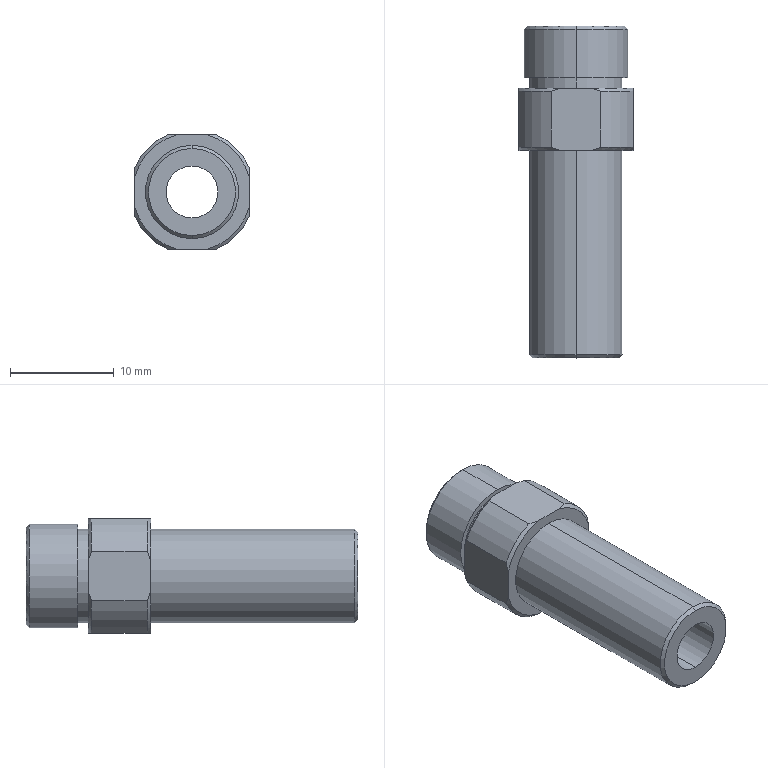Part | SolidWorks | features Chamfer 5, ICE 4, HoleWzd 3, RevCut 2, Extrusion 1 | 1 solid | 33 faces | box 11 x 32 x 11 mm | volume 1736 mm3 | cone 12 | cylinder 12 | plane 9 | commonest cylinder face diameters 9 x4 12 x4 5 x2 10 x2
STEP:
#1=CARTESIAN_POINT('',(0.,-32.,-4.2));
#2=VERTEX_POINT('',#1);
#3=CARTESIAN_POINT('',(0.,-32.,4.2));
#4=VERTEX_POINT('',#3);
#5=CARTESIAN_POINT('',(0.,-32.,0.));
#6=DIRECTION('',(0.,-1.,0.));
#7=DIRECTION('',(0.,0.,-1.));
#8=AXIS2_PLACEMENT_3D('',#5,#6,#7);
#9=CIRCLE('',#8,4.2);
#10=EDGE_CURVE('',#2,#4,#9,.T.);
#11=ORIENTED_EDGE('',*,*,#10,.F.);
#12=CARTESIAN_POINT('',(0.,-31.7,-4.5));
#13=VERTEX_POINT('',#12);
#14=CARTESIAN_POINT('',(0.,-32.,-4.2));
#15=DIRECTION('',(0.,0.7071,-0.7071));
#16=VECTOR('',#15,1000.);
#17=LINE('',#14,#16);
#18=EDGE_CURVE('',#2,#13,#17,.T.);
#19=ORIENTED_EDGE('',*,*,#18,.T.);
#20=CARTESIAN_POINT('',(0.,-31.7,4.5));
#21=VERTEX_POINT('',#20);
#22=CARTESIAN_POINT('',(0.,-31.7,0.));
#23=DIRECTION('',(0.,1.,0.));
#24=DIRECTION('',(0.,0.,-1.));
#25=AXIS2_PLACEMENT_3D('',#22,#23,#24);
#26=CIRCLE('',#25,4.5);
#27=EDGE_CURVE('',#21,#13,#26,.T.);
#28=ORIENTED_EDGE('',*,*,#27,.F.);
#29=CARTESIAN_POINT('',(0.,-32.,4.2));
#30=DIRECTION('',(0.,0.7071,0.7071));
#31=VECTOR('',#30,1000.);
#32=LINE('',#29,#31);
#33=EDGE_CURVE('',#4,#21,#32,.T.);
#34=ORIENTED_EDGE('',*,*,#33,.F.);
#35=EDGE_LOOP('',(#11,#19,#28,#34));
#36=FACE_OUTER_BOUND('',#35,.T.);
#37=CARTESIAN_POINT('',(0.,-32.,0.));
#38=DIRECTION('',(0.,1.,0.));
#39=DIRECTION('',(0.,0.,1.));
#40=AXIS2_PLACEMENT_3D('',#37,#38,#39);
#41=CONICAL_SURFACE('',#40,4.2,0.7854);
#42=ADVANCED_FACE('',(#36),#41,.T.);
#43=CARTESIAN_POINT('',(0.,-5.,-4.5));
#44=VERTEX_POINT('',#43);
#45=CARTESIAN_POINT('',(0.,-5.,4.5));
#46=VERTEX_POINT('',#45);
#47=CARTESIAN_POINT('',(0.,-5.,0.));
#48=DIRECTION('',(0.,-1.,0.));
#49=DIRECTION('',(0.,0.,-1.));
#50=AXIS2_PLACEMENT_3D('',#47,#48,#49);
#51=CIRCLE('',#50,4.5);
#52=EDGE_CURVE('',#44,#46,#51,.T.);
#53=ORIENTED_EDGE('',*,*,#52,.T.);
#54=CARTESIAN_POINT('',(0.,-6.,4.5));
#55=VERTEX_POINT('',#54);
#56=CARTESIAN_POINT('',(0.,-6.,4.5));
#57=DIRECTION('',(0.,-1.,0.));
#58=VECTOR('',#57,1000.);
#59=LINE('',#56,#58);
#60=EDGE_CURVE('',#46,#55,#59,.T.);
#61=ORIENTED_EDGE('',*,*,#60,.T.);
#62=CARTESIAN_POINT('',(0.,-6.,-4.5));
#63=VERTEX_POINT('',#62);
#64=CARTESIAN_POINT('',(0.,-6.,0.));
#65=DIRECTION('',(0.,-1.,0.));
#66=DIRECTION('',(0.,0.,-1.));
#67=AXIS2_PLACEMENT_3D('',#64,#65,#66);
#68=CIRCLE('',#67,4.5);
#69=EDGE_CURVE('',#63,#55,#68,.T.);
#70=ORIENTED_EDGE('',*,*,#69,.F.);
#71=CARTESIAN_POINT('',(0.,-6.,-4.5));
#72=DIRECTION('',(0.,-1.,0.));
#73=VECTOR('',#72,1000.);
#74=LINE('',#71,#73);
#75=EDGE_CURVE('',#44,#63,#74,.T.);
#76=ORIENTED_EDGE('',*,*,#75,.F.);
#77=EDGE_LOOP('',(#53,#61,#70,#76));
#78=FACE_OUTER_BOUND('',#77,.T.);
#79=CARTESIAN_POINT('',(0.,-6.,0.));
#80=DIRECTION('',(0.,-1.,0.));
#81=DIRECTION('',(0.,0.,-1.));
#82=AXIS2_PLACEMENT_3D('',#79,#80,#81);
#83=CYLINDRICAL_SURFACE('',#82,4.5);
#84=ADVANCED_FACE('',(#78),#83,.T.);
#85=CARTESIAN_POINT('',(0.,-32.,2.5));
#86=VERTEX_POINT('',#85);
#87=CARTESIAN_POINT('',(0.,-32.,-2.5));
#88=VERTEX_POINT('',#87);
#89=CARTESIAN_POINT('',(0.,-32.,0.));
#90=DIRECTION('',(0.,-1.,0.));
#91=DIRECTION('',(0.,0.,-1.));
#92=AXIS2_PLACEMENT_3D('',#89,#90,#91);
#93=CIRCLE('',#92,2.5);
#94=EDGE_CURVE('',#86,#88,#93,.T.);
#95=ORIENTED_EDGE('',*,*,#94,.T.);
#96=CARTESIAN_POINT('',(0.,0.,-2.5));
#97=VERTEX_POINT('',#96);
#98=CARTESIAN_POINT('',(0.,0.,-2.5));
#99=DIRECTION('',(0.,1.,0.));
#100=VECTOR('',#99,1000.);
#101=LINE('',#98,#100);
#102=EDGE_CURVE('',#88,#97,#101,.T.);
#103=ORIENTED_EDGE('',*,*,#102,.T.);
#104=CARTESIAN_POINT('',(0.,0.,2.5));
#105=VERTEX_POINT('',#104);
#106=CARTESIAN_POINT('',(0.,0.,0.));
#107=DIRECTION('',(0.,1.,0.));
#108=DIRECTION('',(0.,0.,1.));
#109=AXIS2_PLACEMENT_3D('',#106,#107,#108);
#110=CIRCLE('',#109,2.5);
#111=EDGE_CURVE('',#97,#105,#110,.T.);
#112=ORIENTED_EDGE('',*,*,#111,.T.);
#113=CARTESIAN_POINT('',(0.,0.,2.5));
#114=DIRECTION('',(0.,1.,0.));
#115=VECTOR('',#114,1000.);
#116=LINE('',#113,#115);
#117=EDGE_CURVE('',#86,#105,#116,.T.);
#118=ORIENTED_EDGE('',*,*,#117,.F.);
#119=EDGE_LOOP('',(#95,#103,#112,#118));
#120=FACE_OUTER_BOUND('',#119,.T.);
#121=CARTESIAN_POINT('',(0.,0.,0.));
#122=DIRECTION('',(0.,1.,0.));
#123=DIRECTION('',(0.,0.,1.));
#124=AXIS2_PLACEMENT_3D('',#121,#122,#123);
#125=CYLINDRICAL_SURFACE('',#124,2.5);
#126=ADVANCED_FACE('',(#120),#125,.F.);
#127=CARTESIAN_POINT('',(0.,0.,4.7));
#128=VERTEX_POINT('',#127);
#129=CARTESIAN_POINT('',(0.,0.,-4.7));
#130=VERTEX_POINT('',#129);
#131=CARTESIAN_POINT('',(0.,0.,0.));
#132=DIRECTION('',(0.,1.,0.));
#133=DIRECTION('',(0.,0.,1.));
#134=AXIS2_PLACEMENT_3D('',#131,#132,#133);
#135=CIRCLE('',#134,4.7);
#136=EDGE_CURVE('',#128,#130,#135,.T.);
#137=ORIENTED_EDGE('',*,*,#136,.F.);
#138=CARTESIAN_POINT('',(0.,-0.3,5.));
#139=VERTEX_POINT('',#138);
#140=CARTESIAN_POINT('',(0.,0.,4.7));
#141=DIRECTION('',(0.,-0.7071,0.7071));
#142=VECTOR('',#141,1000.);
#143=LINE('',#140,#142);
#144=EDGE_CURVE('',#128,#139,#143,.T.);
#145=ORIENTED_EDGE('',*,*,#144,.T.);
#146=CARTESIAN_POINT('',(0.,-0.3,-5.));
#147=VERTEX_POINT('',#146);
#148=CARTESIAN_POINT('',(0.,-0.3,0.));
#149=DIRECTION('',(0.,-1.,0.));
#150=DIRECTION('',(0.,0.,1.));
#151=AXIS2_PLACEMENT_3D('',#148,#149,#150);
#152=CIRCLE('',#151,5.);
#153=EDGE_CURVE('',#147,#139,#152,.T.);
#154=ORIENTED_EDGE('',*,*,#153,.F.);
#155=CARTESIAN_POINT('',(0.,0.,-4.7));
#156=DIRECTION('',(0.,-0.7071,-0.7071));
#157=VECTOR('',#156,1000.);
#158=LINE('',#155,#157);
#159=EDGE_CURVE('',#130,#147,#158,.T.);
#160=ORIENTED_EDGE('',*,*,#159,.F.);
#161=EDGE_LOOP('',(#137,#145,#154,#160));
#162=FACE_OUTER_BOUND('',#161,.T.);
#163=CARTESIAN_POINT('',(0.,0.,0.));
#164=DIRECTION('',(0.,-1.,0.));
#165=DIRECTION('',(0.,0.,-1.));
#166=AXIS2_PLACEMENT_3D('',#163,#164,#165);
#167=CONICAL_SURFACE('',#166,4.7,0.7854);
#168=ADVANCED_FACE('',(#162),#167,.T.);
#169=ORIENTED_EDGE('',*,*,#27,.T.);
#170=CARTESIAN_POINT('',(0.,-12.,-4.5));
#171=VERTEX_POINT('',#170);
#172=CARTESIAN_POINT('',(0.,-32.,-4.5));
#173=DIRECTION('',(0.,1.,0.));
#174=VECTOR('',#173,1000.);
#175=LINE('',#172,#174);
#176=EDGE_CURVE('',#13,#171,#175,.T.);
#177=ORIENTED_EDGE('',*,*,#176,.T.);
#178=CARTESIAN_POINT('',(0.,-12.,4.5));
#179=VERTEX_POINT('',#178);
#180=CARTESIAN_POINT('',(0.,-12.,0.));
#181=DIRECTION('',(0.,-1.,0.));
#182=DIRECTION('',(0.,0.,-1.));
#183=AXIS2_PLACEMENT_3D('',#180,#181,#182);
#184=CIRCLE('',#183,4.5);
#185=EDGE_CURVE('',#171,#179,#184,.T.);
#186=ORIENTED_EDGE('',*,*,#185,.T.);
#187=CARTESIAN_POINT('',(0.,-32.,4.5));
#188=DIRECTION('',(0.,1.,0.));
#189=VECTOR('',#188,1000.);
#190=LINE('',#187,#189);
#191=EDGE_CURVE('',#21,#179,#190,.T.);
#192=ORIENTED_EDGE('',*,*,#191,.F.);
#193=EDGE_LOOP('',(#169,#177,#186,#192));
#194=FACE_OUTER_BOUND('',#193,.T.);
#195=CARTESIAN_POINT('',(0.,-32.,0.));
#196=DIRECTION('',(0.,1.,0.));
#197=DIRECTION('',(0.,0.,1.));
#198=AXIS2_PLACEMENT_3D('',#195,#196,#197);
#199=CYLINDRICAL_SURFACE('',#198,4.5);
#200=ADVANCED_FACE('',(#194),#199,.T.);
#201=CARTESIAN_POINT('',(0.,-5.,5.));
#202=VERTEX_POINT('',#201);
#203=CARTESIAN_POINT('',(0.,-5.,-5.));
#204=VERTEX_POINT('',#203);
#205=CARTESIAN_POINT('',(0.,-5.,0.));
#206=DIRECTION('',(0.,1.,0.));
#207=DIRECTION('',(0.,0.,-1.));
#208=AXIS2_PLACEMENT_3D('',#205,#206,#207);
#209=CIRCLE('',#208,5.);
#210=EDGE_CURVE('',#202,#204,#209,.T.);
#211=ORIENTED_EDGE('',*,*,#210,.T.);
#212=CARTESIAN_POINT('',(0.,-6.,-5.));
#213=DIRECTION('',(0.,1.,0.));
#214=VECTOR('',#213,1000.);
#215=LINE('',#212,#214);
#216=EDGE_CURVE('',#204,#147,#215,.T.);
#217=ORIENTED_EDGE('',*,*,#216,.T.);
#218=ORIENTED_EDGE('',*,*,#153,.T.);
#219=CARTESIAN_POINT('',(0.,-6.,5.));
#220=DIRECTION('',(0.,1.,0.));
#221=VECTOR('',#220,1000.);
#222=LINE('',#219,#221);
#223=EDGE_CURVE('',#202,#139,#222,.T.);
#224=ORIENTED_EDGE('',*,*,#223,.F.);
#225=EDGE_LOOP('',(#211,#217,#218,#224));
#226=FACE_OUTER_BOUND('',#225,.T.);
#227=CARTESIAN_POINT('',(0.,-6.,0.));
#228=DIRECTION('',(0.,1.,0.));
#229=DIRECTION('',(0.,0.,1.));
#230=AXIS2_PLACEMENT_3D('',#227,#228,#229);
#231=CYLINDRICAL_SURFACE('',#230,5.);
#232=ADVANCED_FACE('',(#226),#231,.T.);
#233=CARTESIAN_POINT('',(-2.398,-6.3,-5.5));
#234=VERTEX_POINT('',#233);
#235=CARTESIAN_POINT('',(-1.497,-6.,-5.5));
#236=VERTEX_POINT('',#235);
#237=CARTESIAN_POINT('',(-2.398,-6.3,-5.5));
#238=CARTESIAN_POINT('',(-2.104,-6.182,-5.5));
#239=CARTESIAN_POINT('',(-1.804,-6.081,-5.5));
#240=CARTESIAN_POINT('',(-1.497,-6.,-5.5));
#241=B_SPLINE_CURVE_WITH_KNOTS('',3,(#237,#238,#239,#240),.UNSPECIFIED.,.F.,.F.,(4,4),(0.01116,0.01211),.UNSPECIFIED.);
#242=EDGE_CURVE('',#234,#236,#241,.T.);
#243=ORIENTED_EDGE('',*,*,#242,.F.);
#244=CARTESIAN_POINT('',(-5.5,-6.3,-2.398));
#245=VERTEX_POINT('',#244);
#246=CARTESIAN_POINT('',(0.,-6.3,0.));
#247=DIRECTION('',(0.,-1.,0.));
#248=DIRECTION('',(0.,0.,-1.));
#249=AXIS2_PLACEMENT_3D('',#246,#247,#248);
#250=CIRCLE('',#249,6.);
#251=EDGE_CURVE('',#245,#234,#250,.T.);
#252=ORIENTED_EDGE('',*,*,#251,.F.);
#253=CARTESIAN_POINT('',(-5.5,-6.,-1.497));
#254=VERTEX_POINT('',#253);
#255=CARTESIAN_POINT('',(-5.5,-6.,-1.497));
#256=CARTESIAN_POINT('',(-5.5,-6.08,-1.802));
#257=CARTESIAN_POINT('',(-5.5,-6.182,-2.102));
#258=CARTESIAN_POINT('',(-5.5,-6.3,-2.398));
#259=B_SPLINE_CURVE_WITH_KNOTS('',3,(#255,#256,#257,#258),.UNSPECIFIED.,.F.,.F.,(4,4),(0.01603,0.01698),.UNSPECIFIED.);
#260=EDGE_CURVE('',#254,#245,#259,.T.);
#261=ORIENTED_EDGE('',*,*,#260,.F.);
#262=CARTESIAN_POINT('',(0.,-6.,0.));
#263=DIRECTION('',(0.,1.,0.));
#264=DIRECTION('',(0.,0.,-1.));
#265=AXIS2_PLACEMENT_3D('',#262,#263,#264);
#266=CIRCLE('',#265,5.7);
#267=EDGE_CURVE('',#236,#254,#266,.T.);
#268=ORIENTED_EDGE('',*,*,#267,.F.);
#269=EDGE_LOOP('',(#243,#252,#261,#268));
#270=FACE_OUTER_BOUND('',#269,.T.);
#271=CARTESIAN_POINT('',(0.,-6.3,0.));
#272=DIRECTION('',(0.,-1.,0.));
#273=DIRECTION('',(0.,0.,-1.));
#274=AXIS2_PLACEMENT_3D('',#271,#272,#273);
#275=CONICAL_SURFACE('',#274,6.,0.7854);
#276=ADVANCED_FACE('',(#270),#275,.T.);
#277=CARTESIAN_POINT('',(5.5,-11.7,-2.398));
#278=VERTEX_POINT('',#277);
#279=CARTESIAN_POINT('',(2.398,-11.7,-5.5));
#280=VERTEX_POINT('',#279);
#281=CARTESIAN_POINT('',(0.,-11.7,0.));
#282=DIRECTION('',(0.,1.,0.));
#283=DIRECTION('',(0.,0.,-1.));
#284=AXIS2_PLACEMENT_3D('',#281,#282,#283);
#285=CIRCLE('',#284,6.);
#286=EDGE_CURVE('',#278,#280,#285,.T.);
#287=ORIENTED_EDGE('',*,*,#286,.T.);
#288=CARTESIAN_POINT('',(2.398,-6.3,-5.5));
#289=VERTEX_POINT('',#288);
#290=CARTESIAN_POINT('',(2.398,-12.,-5.5));
#291=DIRECTION('',(0.,1.,0.));
#292=VECTOR('',#291,1000.);
#293=LINE('',#290,#292);
#294=EDGE_CURVE('',#280,#289,#293,.T.);
#295=ORIENTED_EDGE('',*,*,#294,.T.);
#296=CARTESIAN_POINT('',(5.5,-6.3,-2.398));
#297=VERTEX_POINT('',#296);
#298=CARTESIAN_POINT('',(0.,-6.3,0.));
#299=DIRECTION('',(0.,-1.,0.));
#300=DIRECTION('',(0.,0.,-1.));
#301=AXIS2_PLACEMENT_3D('',#298,#299,#300);
#302=CIRCLE('',#301,6.);
#303=EDGE_CURVE('',#289,#297,#302,.T.);
#304=ORIENTED_EDGE('',*,*,#303,.T.);
#305=CARTESIAN_POINT('',(5.5,-12.,-2.398));
#306=DIRECTION('',(0.,-1.,0.));
#307=VECTOR('',#306,1000.);
#308=LINE('',#305,#307);
#309=EDGE_CURVE('',#297,#278,#308,.T.);
#310=ORIENTED_EDGE('',*,*,#309,.T.);
#311=EDGE_LOOP('',(#287,#295,#304,#310));
#312=FACE_OUTER_BOUND('',#311,.T.);
#313=CARTESIAN_POINT('',(0.,-12.,0.));
#314=DIRECTION('',(0.,1.,0.));
#315=DIRECTION('',(0.,0.,1.));
#316=AXIS2_PLACEMENT_3D('',#313,#314,#315);
#317=CYLINDRICAL_SURFACE('',#316,6.);
#318=ADVANCED_FACE('',(#312),#317,.T.);
#319=CARTESIAN_POINT('',(1.497,-12.,-5.5));
#320=VERTEX_POINT('',#319);
#321=CARTESIAN_POINT('',(2.398,-11.7,-5.5));
#322=CARTESIAN_POINT('',(2.104,-11.818,-5.5));
#323=CARTESIAN_POINT('',(1.804,-11.919,-5.5));
#324=CARTESIAN_POINT('',(1.497,-12.,-5.5));
#325=B_SPLINE_CURVE_WITH_KNOTS('',3,(#321,#322,#323,#324),.UNSPECIFIED.,.F.,.F.,(4,4),(0.01116,0.01211),.UNSPECIFIED.);
#326=EDGE_CURVE('',#280,#320,#325,.T.);
#327=ORIENTED_EDGE('',*,*,#326,.F.);
#328=ORIENTED_EDGE('',*,*,#286,.F.);
#329=CARTESIAN_POINT('',(5.5,-12.,-1.497));
#330=VERTEX_POINT('',#329);
#331=CARTESIAN_POINT('',(5.5,-12.,-1.497));
#332=CARTESIAN_POINT('',(5.5,-11.92,-1.802));
#333=CARTESIAN_POINT('',(5.5,-11.818,-2.102));
#334=CARTESIAN_POINT('',(5.5,-11.7,-2.398));
#335=B_SPLINE_CURVE_WITH_KNOTS('',3,(#331,#332,#333,#334),.UNSPECIFIED.,.F.,.F.,(4,4),(0.01603,0.01698),.UNSPECIFIED.);
#336=EDGE_CURVE('',#330,#278,#335,.T.);
#337=ORIENTED_EDGE('',*,*,#336,.F.);
#338=CARTESIAN_POINT('',(0.,-12.,0.));
#339=DIRECTION('',(0.,-1.,0.));
#340=DIRECTION('',(0.,0.,-1.));
#341=AXIS2_PLACEMENT_3D('',#338,#339,#340);
#342=CIRCLE('',#341,5.7);
#343=EDGE_CURVE('',#320,#330,#342,.T.);
#344=ORIENTED_EDGE('',*,*,#343,.F.);
#345=EDGE_LOOP('',(#327,#328,#337,#344));
#346=FACE_OUTER_BOUND('',#345,.T.);
#347=CARTESIAN_POINT('',(0.,-12.,0.));
#348=DIRECTION('',(0.,1.,0.));
#349=DIRECTION('',(0.,0.,1.));
#350=AXIS2_PLACEMENT_3D('',#347,#348,#349);
#351=CONICAL_SURFACE('',#350,5.7,0.7854);
#352=ADVANCED_FACE('',(#346),#351,.T.);
#353=CARTESIAN_POINT('',(-5.5,-11.7,2.398));
#354=VERTEX_POINT('',#353);
#355=CARTESIAN_POINT('',(-2.398,-11.7,5.5));
#356=VERTEX_POINT('',#355);
#357=CARTESIAN_POINT('',(0.,-11.7,0.));
#358=DIRECTION('',(0.,1.,0.));
#359=DIRECTION('',(0.,0.,-1.));
#360=AXIS2_PLACEMENT_3D('',#357,#358,#359);
#361=CIRCLE('',#360,6.);
#362=EDGE_CURVE('',#354,#356,#361,.T.);
#363=ORIENTED_EDGE('',*,*,#362,.T.);
#364=CARTESIAN_POINT('',(-2.398,-6.3,5.5));
#365=VERTEX_POINT('',#364);
#366=CARTESIAN_POINT('',(-2.398,-12.,5.5));
#367=DIRECTION('',(0.,1.,0.));
#368=VECTOR('',#367,1000.);
#369=LINE('',#366,#368);
#370=EDGE_CURVE('',#356,#365,#369,.T.);
#371=ORIENTED_EDGE('',*,*,#370,.T.);
#372=CARTESIAN_POINT('',(-5.5,-6.3,2.398));
#373=VERTEX_POINT('',#372);
#374=CARTESIAN_POINT('',(0.,-6.3,0.));
#375=DIRECTION('',(0.,-1.,0.));
#376=DIRECTION('',(0.,0.,-1.));
#377=AXIS2_PLACEMENT_3D('',#374,#375,#376);
#378=CIRCLE('',#377,6.);
#379=EDGE_CURVE('',#365,#373,#378,.T.);
#380=ORIENTED_EDGE('',*,*,#379,.T.);
#381=CARTESIAN_POINT('',(-5.5,-12.,2.398));
#382=DIRECTION('',(0.,-1.,0.));
#383=VECTOR('',#382,1000.);
#384=LINE('',#381,#383);
#385=EDGE_CURVE('',#373,#354,#384,.T.);
#386=ORIENTED_EDGE('',*,*,#385,.T.);
#387=EDGE_LOOP('',(#363,#371,#380,#386));
#388=FACE_OUTER_BOUND('',#387,.T.);
#389=CARTESIAN_POINT('',(0.,-12.,0.));
#390=DIRECTION('',(0.,1.,0.));
#391=DIRECTION('',(0.,0.,1.));
#392=AXIS2_PLACEMENT_3D('',#389,#390,#391);
#393=CYLINDRICAL_SURFACE('',#392,6.);
#394=ADVANCED_FACE('',(#388),#393,.T.);
#395=CARTESIAN_POINT('',(-1.497,-12.,5.5));
#396=VERTEX_POINT('',#395);
#397=CARTESIAN_POINT('',(-2.398,-11.7,5.5));
#398=CARTESIAN_POINT('',(-2.104,-11.818,5.5));
#399=CARTESIAN_POINT('',(-1.804,-11.919,5.5));
#400=CARTESIAN_POINT('',(-1.497,-12.,5.5));
#401=B_SPLINE_CURVE_WITH_KNOTS('',3,(#397,#398,#399,#400),.UNSPECIFIED.,.F.,.F.,(4,4),(0.01116,0.01211),.UNSPECIFIED.);
#402=EDGE_CURVE('',#356,#396,#401,.T.);
#403=ORIENTED_EDGE('',*,*,#402,.F.);
#404=ORIENTED_EDGE('',*,*,#362,.F.);
#405=CARTESIAN_POINT('',(-5.5,-12.,1.497));
#406=VERTEX_POINT('',#405);
#407=CARTESIAN_POINT('',(-5.5,-12.,1.497));
#408=CARTESIAN_POINT('',(-5.5,-11.92,1.802));
#409=CARTESIAN_POINT('',(-5.5,-11.818,2.102));
#410=CARTESIAN_POINT('',(-5.5,-11.7,2.398));
#411=B_SPLINE_CURVE_WITH_KNOTS('',3,(#407,#408,#409,#410),.UNSPECIFIED.,.F.,.F.,(4,4),(0.01603,0.01698),.UNSPECIFIED.);
#412=EDGE_CURVE('',#406,#354,#411,.T.);
#413=ORIENTED_EDGE('',*,*,#412,.F.);
#414=CARTESIAN_POINT('',(0.,-12.,0.));
#415=DIRECTION('',(0.,-1.,0.));
#416=DIRECTION('',(0.,0.,-1.));
#417=AXIS2_PLACEMENT_3D('',#414,#415,#416);
#418=CIRCLE('',#417,5.7);
#419=EDGE_CURVE('',#396,#406,#418,.T.);
#420=ORIENTED_EDGE('',*,*,#419,.F.);
#421=EDGE_LOOP('',(#403,#404,#413,#420));
#422=FACE_OUTER_BOUND('',#421,.T.);
#423=CARTESIAN_POINT('',(0.,-12.,0.));
#424=DIRECTION('',(0.,1.,0.));
#425=DIRECTION('',(0.,0.,1.));
#426=AXIS2_PLACEMENT_3D('',#423,#424,#425);
#427=CONICAL_SURFACE('',#426,5.7,0.7854);
#428=ADVANCED_FACE('',(#422),#427,.T.);
#429=CARTESIAN_POINT('',(2.398,-6.3,5.5));
#430=VERTEX_POINT('',#429);
#431=CARTESIAN_POINT('',(1.497,-6.,5.5));
#432=VERTEX_POINT('',#431);
#433=CARTESIAN_POINT('',(2.398,-6.3,5.5));
#434=CARTESIAN_POINT('',(2.104,-6.182,5.5));
#435=CARTESIAN_POINT('',(1.804,-6.081,5.5));
#436=CARTESIAN_POINT('',(1.497,-6.,5.5));
#437=B_SPLINE_CURVE_WITH_KNOTS('',3,(#433,#434,#435,#436),.UNSPECIFIED.,.F.,.F.,(4,4),(0.01116,0.01211),.UNSPECIFIED.);
#438=EDGE_CURVE('',#430,#432,#437,.T.);
#439=ORIENTED_EDGE('',*,*,#438,.F.);
#440=CARTESIAN_POINT('',(5.5,-6.3,2.398));
#441=VERTEX_POINT('',#440);
#442=CARTESIAN_POINT('',(0.,-6.3,0.));
#443=DIRECTION('',(0.,-1.,0.));
#444=DIRECTION('',(0.,0.,-1.));
#445=AXIS2_PLACEMENT_3D('',#442,#443,#444);
#446=CIRCLE('',#445,6.);
#447=EDGE_CURVE('',#441,#430,#446,.T.);
#448=ORIENTED_EDGE('',*,*,#447,.F.);
#449=CARTESIAN_POINT('',(5.5,-6.,1.497));
#450=VERTEX_POINT('',#449);
#451=CARTESIAN_POINT('',(5.5,-6.,1.497));
#452=CARTESIAN_POINT('',(5.5,-6.08,1.802));
#453=CARTESIAN_POINT('',(5.5,-6.182,2.102));
#454=CARTESIAN_POINT('',(5.5,-6.3,2.398));
#455=B_SPLINE_CURVE_WITH_KNOTS('',3,(#451,#452,#453,#454),.UNSPECIFIED.,.F.,.F.,(4,4),(0.01603,0.01698),.UNSPECIFIED.);
#456=EDGE_CURVE('',#450,#441,#455,.T.);
#457=ORIENTED_EDGE('',*,*,#456,.F.);
#458=CARTESIAN_POINT('',(0.,-6.,0.));
#459=DIRECTION('',(0.,1.,0.));
#460=DIRECTION('',(0.,0.,-1.));
#461=AXIS2_PLACEMENT_3D('',#458,#459,#460);
#462=CIRCLE('',#461,5.7);
#463=EDGE_CURVE('',#432,#450,#462,.T.);
#464=ORIENTED_EDGE('',*,*,#463,.F.);
#465=EDGE_LOOP('',(#439,#448,#457,#464));
#466=FACE_OUTER_BOUND('',#465,.T.);
#467=CARTESIAN_POINT('',(0.,-6.3,0.));
#468=DIRECTION('',(0.,-1.,0.));
#469=DIRECTION('',(0.,0.,-1.));
#470=AXIS2_PLACEMENT_3D('',#467,#468,#469);
#471=CONICAL_SURFACE('',#470,6.,0.7854);
#472=ADVANCED_FACE('',(#466),#471,.T.);
#473=ORIENTED_EDGE('',*,*,#216,.F.);
#474=CARTESIAN_POINT('',(0.,-5.,0.));
#475=DIRECTION('',(0.,1.,0.));
#476=DIRECTION('',(0.,0.,-1.));
#477=AXIS2_PLACEMENT_3D('',#474,#475,#476);
#478=CIRCLE('',#477,5.);
#479=EDGE_CURVE('',#204,#202,#478,.T.);
#480=ORIENTED_EDGE('',*,*,#479,.T.);
#481=ORIENTED_EDGE('',*,*,#223,.T.);
#482=CARTESIAN_POINT('',(0.,-0.3,0.));
#483=DIRECTION('',(0.,-1.,0.));
#484=DIRECTION('',(0.,0.,1.));
#485=AXIS2_PLACEMENT_3D('',#482,#483,#484);
#486=CIRCLE('',#485,5.);
#487=EDGE_CURVE('',#139,#147,#486,.T.);
#488=ORIENTED_EDGE('',*,*,#487,.T.);
#489=EDGE_LOOP('',(#473,#480,#481,#488));
#490=FACE_OUTER_BOUND('',#489,.T.);
#491=CARTESIAN_POINT('',(0.,-6.,0.));
#492=DIRECTION('',(0.,1.,0.));
#493=DIRECTION('',(0.,0.,1.));
#494=AXIS2_PLACEMENT_3D('',#491,#492,#493);
#495=CYLINDRICAL_SURFACE('',#494,5.);
#496=ADVANCED_FACE('',(#490),#495,.T.);
#497=ORIENTED_EDGE('',*,*,#447,.T.);
#498=CARTESIAN_POINT('',(2.398,-11.7,5.5));
#499=VERTEX_POINT('',#498);
#500=CARTESIAN_POINT('',(2.398,-12.,5.5));
#501=DIRECTION('',(0.,-1.,0.));
#502=VECTOR('',#501,1000.);
#503=LINE('',#500,#502);
#504=EDGE_CURVE('',#430,#499,#503,.T.);
#505=ORIENTED_EDGE('',*,*,#504,.T.);
#506=CARTESIAN_POINT('',(5.5,-11.7,2.398));
#507=VERTEX_POINT('',#506);
#508=CARTESIAN_POINT('',(0.,-11.7,0.));
#509=DIRECTION('',(0.,1.,0.));
#510=DIRECTION('',(0.,0.,-1.));
#511=AXIS2_PLACEMENT_3D('',#508,#509,#510);
#512=CIRCLE('',#511,6.);
#513=EDGE_CURVE('',#499,#507,#512,.T.);
#514=ORIENTED_EDGE('',*,*,#513,.T.);
#515=CARTESIAN_POINT('',(5.5,-12.,2.398));
#516=DIRECTION('',(0.,1.,0.));
#517=VECTOR('',#516,1000.);
#518=LINE('',#515,#517);
#519=EDGE_CURVE('',#507,#441,#518,.T.);
#520=ORIENTED_EDGE('',*,*,#519,.T.);
#521=EDGE_LOOP('',(#497,#505,#514,#520));
#522=FACE_OUTER_BOUND('',#521,.T.);
#523=CARTESIAN_POINT('',(0.,-12.,0.));
#524=DIRECTION('',(0.,1.,0.));
#525=DIRECTION('',(0.,0.,1.));
#526=AXIS2_PLACEMENT_3D('',#523,#524,#525);
#527=CYLINDRICAL_SURFACE('',#526,6.);
#528=ADVANCED_FACE('',(#522),#527,.T.);
#529=CARTESIAN_POINT('',(1.497,-12.,5.5));
#530=VERTEX_POINT('',#529);
#531=CARTESIAN_POINT('',(1.497,-12.,5.5));
#532=CARTESIAN_POINT('',(1.804,-11.919,5.5));
#533=CARTESIAN_POINT('',(2.104,-11.818,5.5));
#534=CARTESIAN_POINT('',(2.398,-11.7,5.5));
#535=B_SPLINE_CURVE_WITH_KNOTS('',3,(#531,#532,#533,#534),.UNSPECIFIED.,.F.,.F.,(4,4),(0.01514,0.01609),.UNSPECIFIED.);
#536=EDGE_CURVE('',#530,#499,#535,.T.);
#537=ORIENTED_EDGE('',*,*,#536,.F.);
#538=CARTESIAN_POINT('',(5.5,-12.,1.497));
#539=VERTEX_POINT('',#538);
#540=CARTESIAN_POINT('',(0.,-12.,0.));
#541=DIRECTION('',(0.,-1.,0.));
#542=DIRECTION('',(0.,0.,-1.));
#543=AXIS2_PLACEMENT_3D('',#540,#541,#542);
#544=CIRCLE('',#543,5.7);
#545=EDGE_CURVE('',#539,#530,#544,.T.);
#546=ORIENTED_EDGE('',*,*,#545,.F.);
#547=CARTESIAN_POINT('',(5.5,-11.7,2.398));
#548=CARTESIAN_POINT('',(5.5,-11.817,2.105));
#549=CARTESIAN_POINT('',(5.5,-11.919,1.805));
#550=CARTESIAN_POINT('',(5.5,-12.,1.497));
#551=B_SPLINE_CURVE_WITH_KNOTS('',3,(#547,#548,#549,#550),.UNSPECIFIED.,.F.,.F.,(4,4),(0.01206,0.01301),.UNSPECIFIED.);
#552=EDGE_CURVE('',#507,#539,#551,.T.);
#553=ORIENTED_EDGE('',*,*,#552,.F.);
#554=ORIENTED_EDGE('',*,*,#513,.F.);
#555=EDGE_LOOP('',(#537,#546,#553,#554));
#556=FACE_OUTER_BOUND('',#555,.T.);
#557=CARTESIAN_POINT('',(0.,-12.,0.));
#558=DIRECTION('',(0.,1.,0.));
#559=DIRECTION('',(0.,0.,1.));
#560=AXIS2_PLACEMENT_3D('',#557,#558,#559);
#561=CONICAL_SURFACE('',#560,5.7,0.7854);
#562=ADVANCED_FACE('',(#556),#561,.T.);
#563=CARTESIAN_POINT('',(1.497,-6.,-5.5));
#564=VERTEX_POINT('',#563);
#565=CARTESIAN_POINT('',(1.497,-6.,-5.5));
#566=CARTESIAN_POINT('',(1.804,-6.081,-5.5));
#567=CARTESIAN_POINT('',(2.104,-6.182,-5.5));
#568=CARTESIAN_POINT('',(2.398,-6.3,-5.5));
#569=B_SPLINE_CURVE_WITH_KNOTS('',3,(#565,#566,#567,#568),.UNSPECIFIED.,.F.,.F.,(4,4),(0.01514,0.01609),.UNSPECIFIED.);
#570=EDGE_CURVE('',#564,#289,#569,.T.);
#571=ORIENTED_EDGE('',*,*,#570,.F.);
#572=CARTESIAN_POINT('',(5.5,-6.,-1.497));
#573=VERTEX_POINT('',#572);
#574=CARTESIAN_POINT('',(0.,-6.,0.));
#575=DIRECTION('',(0.,1.,0.));
#576=DIRECTION('',(0.,0.,-1.));
#577=AXIS2_PLACEMENT_3D('',#574,#575,#576);
#578=CIRCLE('',#577,5.7);
#579=EDGE_CURVE('',#573,#564,#578,.T.);
#580=ORIENTED_EDGE('',*,*,#579,.F.);
#581=CARTESIAN_POINT('',(5.5,-6.3,-2.398));
#582=CARTESIAN_POINT('',(5.5,-6.183,-2.105));
#583=CARTESIAN_POINT('',(5.5,-6.081,-1.805));
#584=CARTESIAN_POINT('',(5.5,-6.,-1.497));
#585=B_SPLINE_CURVE_WITH_KNOTS('',3,(#581,#582,#583,#584),.UNSPECIFIED.,.F.,.F.,(4,4),(0.01206,0.01301),.UNSPECIFIED.);
#586=EDGE_CURVE('',#297,#573,#585,.T.);
#587=ORIENTED_EDGE('',*,*,#586,.F.);
#588=ORIENTED_EDGE('',*,*,#303,.F.);
#589=EDGE_LOOP('',(#571,#580,#587,#588));
#590=FACE_OUTER_BOUND('',#589,.T.);
#591=CARTESIAN_POINT('',(0.,-6.3,0.));
#592=DIRECTION('',(0.,-1.,0.));
#593=DIRECTION('',(0.,0.,-1.));
#594=AXIS2_PLACEMENT_3D('',#591,#592,#593);
#595=CONICAL_SURFACE('',#594,6.,0.7854);
#596=ADVANCED_FACE('',(#590),#595,.T.);
#597=CARTESIAN_POINT('',(-1.497,-12.,-5.5));
#598=VERTEX_POINT('',#597);
#599=CARTESIAN_POINT('',(0.,-12.,-5.5));
#600=DIRECTION('',(-1.,0.,0.));
#601=VECTOR('',#600,1000.);
#602=LINE('',#599,#601);
#603=EDGE_CURVE('',#320,#598,#602,.T.);
#604=ORIENTED_EDGE('',*,*,#603,.F.);
#605=ORIENTED_EDGE('',*,*,#343,.T.);
#606=CARTESIAN_POINT('',(5.5,-12.,0.));
#607=DIRECTION('',(0.,0.,-1.));
#608=VECTOR('',#607,1000.);
#609=LINE('',#606,#608);
#610=EDGE_CURVE('',#539,#330,#609,.T.);
#611=ORIENTED_EDGE('',*,*,#610,.F.);
#612=ORIENTED_EDGE('',*,*,#545,.T.);
#613=CARTESIAN_POINT('',(0.,-12.,5.5));
#614=DIRECTION('',(1.,0.,0.));
#615=VECTOR('',#614,1000.);
#616=LINE('',#613,#615);
#617=EDGE_CURVE('',#396,#530,#616,.T.);
#618=ORIENTED_EDGE('',*,*,#617,.F.);
#619=ORIENTED_EDGE('',*,*,#419,.T.);
#620=CARTESIAN_POINT('',(-5.5,-12.,-1.497));
#621=VERTEX_POINT('',#620);
#622=CARTESIAN_POINT('',(-5.5,-12.,0.));
#623=DIRECTION('',(0.,0.,1.));
#624=VECTOR('',#623,1000.);
#625=LINE('',#622,#624);
#626=EDGE_CURVE('',#621,#406,#625,.T.);
#627=ORIENTED_EDGE('',*,*,#626,.F.);
#628=CARTESIAN_POINT('',(0.,-12.,0.));
#629=DIRECTION('',(0.,-1.,0.));
#630=DIRECTION('',(0.,0.,-1.));
#631=AXIS2_PLACEMENT_3D('',#628,#629,#630);
#632=CIRCLE('',#631,5.7);
#633=EDGE_CURVE('',#621,#598,#632,.T.);
#634=ORIENTED_EDGE('',*,*,#633,.T.);
#635=EDGE_LOOP('',(#604,#605,#611,#612,#618,#619,#627,#634));
#636=FACE_OUTER_BOUND('',#635,.T.);
#637=CARTESIAN_POINT('',(0.,-12.,0.));
#638=DIRECTION('',(0.,-1.,0.));
#639=DIRECTION('',(0.,0.,-1.));
#640=AXIS2_PLACEMENT_3D('',#637,#638,#639);
#641=CIRCLE('',#640,4.5);
#642=EDGE_CURVE('',#179,#171,#641,.T.);
#643=ORIENTED_EDGE('',*,*,#642,.F.);
#644=ORIENTED_EDGE('',*,*,#185,.F.);
#645=EDGE_LOOP('',(#643,#644));
#646=FACE_BOUND('',#645,.T.);
#647=CARTESIAN_POINT('',(0.,-12.,0.));
#648=DIRECTION('',(0.,-1.,0.));
#649=DIRECTION('',(0.,0.,-1.));
#650=AXIS2_PLACEMENT_3D('',#647,#648,#649);
#651=PLANE('',#650);
#652=ADVANCED_FACE('',(#636,#646),#651,.T.);
#653=CARTESIAN_POINT('',(0.,0.,0.));
#654=DIRECTION('',(0.,1.,0.));
#655=DIRECTION('',(0.,0.,1.));
#656=AXIS2_PLACEMENT_3D('',#653,#654,#655);
#657=CIRCLE('',#656,2.5);
#658=EDGE_CURVE('',#105,#97,#657,.T.);
#659=ORIENTED_EDGE('',*,*,#658,.F.);
#660=ORIENTED_EDGE('',*,*,#111,.F.);
#661=EDGE_LOOP('',(#659,#660));
#662=FACE_BOUND('',#661,.T.);
#663=CARTESIAN_POINT('',(0.,0.,0.));
#664=DIRECTION('',(0.,1.,0.));
#665=DIRECTION('',(0.,0.,1.));
#666=AXIS2_PLACEMENT_3D('',#663,#664,#665);
#667=CIRCLE('',#666,4.7);
#668=EDGE_CURVE('',#130,#128,#667,.T.);
#669=ORIENTED_EDGE('',*,*,#668,.T.);
#670=ORIENTED_EDGE('',*,*,#136,.T.);
#671=EDGE_LOOP('',(#669,#670));
#672=FACE_OUTER_BOUND('',#671,.T.);
#673=CARTESIAN_POINT('',(0.,0.,0.));
#674=DIRECTION('',(0.,1.,0.));
#675=DIRECTION('',(0.,0.,1.));
#676=AXIS2_PLACEMENT_3D('',#673,#674,#675);
#677=PLANE('',#676);
#678=ADVANCED_FACE('',(#662,#672),#677,.T.);
#679=ORIENTED_EDGE('',*,*,#251,.T.);
#680=CARTESIAN_POINT('',(-2.398,-11.7,-5.5));
#681=VERTEX_POINT('',#680);
#682=CARTESIAN_POINT('',(-2.398,-12.,-5.5));
#683=DIRECTION('',(0.,-1.,0.));
#684=VECTOR('',#683,1000.);
#685=LINE('',#682,#684);
#686=EDGE_CURVE('',#234,#681,#685,.T.);
#687=ORIENTED_EDGE('',*,*,#686,.T.);
#688=CARTESIAN_POINT('',(-5.5,-11.7,-2.398));
#689=VERTEX_POINT('',#688);
#690=CARTESIAN_POINT('',(0.,-11.7,0.));
#691=DIRECTION('',(0.,1.,0.));
#692=DIRECTION('',(0.,0.,-1.));
#693=AXIS2_PLACEMENT_3D('',#690,#691,#692);
#694=CIRCLE('',#693,6.);
#695=EDGE_CURVE('',#681,#689,#694,.T.);
#696=ORIENTED_EDGE('',*,*,#695,.T.);
#697=CARTESIAN_POINT('',(-5.5,-12.,-2.398));
#698=DIRECTION('',(0.,1.,0.));
#699=VECTOR('',#698,1000.);
#700=LINE('',#697,#699);
#701=EDGE_CURVE('',#689,#245,#700,.T.);
#702=ORIENTED_EDGE('',*,*,#701,.T.);
#703=EDGE_LOOP('',(#679,#687,#696,#702));
#704=FACE_OUTER_BOUND('',#703,.T.);
#705=CARTESIAN_POINT('',(0.,-12.,0.));
#706=DIRECTION('',(0.,1.,0.));
#707=DIRECTION('',(0.,0.,1.));
#708=AXIS2_PLACEMENT_3D('',#705,#706,#707);
#709=CYLINDRICAL_SURFACE('',#708,6.);
#710=ADVANCED_FACE('',(#704),#709,.T.);
#711=ORIENTED_EDGE('',*,*,#579,.T.);
#712=CARTESIAN_POINT('',(0.,-6.,-5.5));
#713=DIRECTION('',(-1.,0.,0.));
#714=VECTOR('',#713,1000.);
#715=LINE('',#712,#714);
#716=EDGE_CURVE('',#564,#236,#715,.T.);
#717=ORIENTED_EDGE('',*,*,#716,.T.);
#718=ORIENTED_EDGE('',*,*,#267,.T.);
#719=CARTESIAN_POINT('',(-5.5,-6.,1.497));
#720=VERTEX_POINT('',#719);
#721=CARTESIAN_POINT('',(-5.5,-6.,0.));
#722=DIRECTION('',(0.,0.,1.));
#723=VECTOR('',#722,1000.);
#724=LINE('',#721,#723);
#725=EDGE_CURVE('',#254,#720,#724,.T.);
#726=ORIENTED_EDGE('',*,*,#725,.T.);
#727=CARTESIAN_POINT('',(-1.497,-6.,5.5));
#728=VERTEX_POINT('',#727);
#729=CARTESIAN_POINT('',(0.,-6.,0.));
#730=DIRECTION('',(0.,1.,0.));
#731=DIRECTION('',(0.,0.,-1.));
#732=AXIS2_PLACEMENT_3D('',#729,#730,#731);
#733=CIRCLE('',#732,5.7);
#734=EDGE_CURVE('',#720,#728,#733,.T.);
#735=ORIENTED_EDGE('',*,*,#734,.T.);
#736=CARTESIAN_POINT('',(0.,-6.,5.5));
#737=DIRECTION('',(1.,0.,0.));
#738=VECTOR('',#737,1000.);
#739=LINE('',#736,#738);
#740=EDGE_CURVE('',#728,#432,#739,.T.);
#741=ORIENTED_EDGE('',*,*,#740,.T.);
#742=ORIENTED_EDGE('',*,*,#463,.T.);
#743=CARTESIAN_POINT('',(5.5,-6.,0.));
#744=DIRECTION('',(0.,0.,-1.));
#745=VECTOR('',#744,1000.);
#746=LINE('',#743,#745);
#747=EDGE_CURVE('',#450,#573,#746,.T.);
#748=ORIENTED_EDGE('',*,*,#747,.T.);
#749=EDGE_LOOP('',(#711,#717,#718,#726,#735,#741,#742,#748));
#750=FACE_OUTER_BOUND('',#749,.T.);
#751=ORIENTED_EDGE('',*,*,#69,.T.);
#752=CARTESIAN_POINT('',(0.,-6.,0.));
#753=DIRECTION('',(0.,-1.,0.));
#754=DIRECTION('',(0.,0.,-1.));
#755=AXIS2_PLACEMENT_3D('',#752,#753,#754);
#756=CIRCLE('',#755,4.5);
#757=EDGE_CURVE('',#55,#63,#756,.T.);
#758=ORIENTED_EDGE('',*,*,#757,.T.);
#759=EDGE_LOOP('',(#751,#758));
#760=FACE_BOUND('',#759,.T.);
#761=CARTESIAN_POINT('',(0.,-6.,0.));
#762=DIRECTION('',(0.,-1.,0.));
#763=DIRECTION('',(0.,0.,-1.));
#764=AXIS2_PLACEMENT_3D('',#761,#762,#763);
#765=PLANE('',#764);
#766=ADVANCED_FACE('',(#750,#760),#765,.F.);
#767=ORIENTED_EDGE('',*,*,#176,.F.);
#768=CARTESIAN_POINT('',(0.,-31.7,0.));
#769=DIRECTION('',(0.,1.,0.));
#770=DIRECTION('',(0.,0.,-1.));
#771=AXIS2_PLACEMENT_3D('',#768,#769,#770);
#772=CIRCLE('',#771,4.5);
#773=EDGE_CURVE('',#13,#21,#772,.T.);
#774=ORIENTED_EDGE('',*,*,#773,.T.);
#775=ORIENTED_EDGE('',*,*,#191,.T.);
#776=ORIENTED_EDGE('',*,*,#642,.T.);
#777=EDGE_LOOP('',(#767,#774,#775,#776));
#778=FACE_OUTER_BOUND('',#777,.T.);
#779=CARTESIAN_POINT('',(0.,-32.,0.));
#780=DIRECTION('',(0.,1.,0.));
#781=DIRECTION('',(0.,0.,1.));
#782=AXIS2_PLACEMENT_3D('',#779,#780,#781);
#783=CYLINDRICAL_SURFACE('',#782,4.5);
#784=ADVANCED_FACE('',(#778),#783,.T.);
#785=CARTESIAN_POINT('',(0.,-32.,0.));
#786=DIRECTION('',(0.,-1.,0.));
#787=DIRECTION('',(0.,0.,-1.));
#788=AXIS2_PLACEMENT_3D('',#785,#786,#787);
#789=CIRCLE('',#788,4.2);
#790=EDGE_CURVE('',#4,#2,#789,.T.);
#791=ORIENTED_EDGE('',*,*,#790,.T.);
#792=ORIENTED_EDGE('',*,*,#10,.T.);
#793=EDGE_LOOP('',(#791,#792));
#794=FACE_OUTER_BOUND('',#793,.T.);
#795=ORIENTED_EDGE('',*,*,#94,.F.);
#796=CARTESIAN_POINT('',(0.,-32.,0.));
#797=DIRECTION('',(0.,-1.,0.));
#798=DIRECTION('',(0.,0.,-1.));
#799=AXIS2_PLACEMENT_3D('',#796,#797,#798);
#800=CIRCLE('',#799,2.5);
#801=EDGE_CURVE('',#88,#86,#800,.T.);
#802=ORIENTED_EDGE('',*,*,#801,.F.);
#803=EDGE_LOOP('',(#795,#802));
#804=FACE_BOUND('',#803,.T.);
#805=CARTESIAN_POINT('',(0.,-32.,0.));
#806=DIRECTION('',(0.,-1.,0.));
#807=DIRECTION('',(0.,0.,-1.));
#808=AXIS2_PLACEMENT_3D('',#805,#806,#807);
#809=PLANE('',#808);
#810=ADVANCED_FACE('',(#794,#804),#809,.T.);
#811=CARTESIAN_POINT('',(-1.497,-12.,-5.5));
#812=CARTESIAN_POINT('',(-1.804,-11.919,-5.5));
#813=CARTESIAN_POINT('',(-2.104,-11.818,-5.5));
#814=CARTESIAN_POINT('',(-2.398,-11.7,-5.5));
#815=B_SPLINE_CURVE_WITH_KNOTS('',3,(#811,#812,#813,#814),.UNSPECIFIED.,.F.,.F.,(4,4),(0.01514,0.01609),.UNSPECIFIED.);
#816=EDGE_CURVE('',#598,#681,#815,.T.);
#817=ORIENTED_EDGE('',*,*,#816,.F.);
#818=ORIENTED_EDGE('',*,*,#633,.F.);
#819=CARTESIAN_POINT('',(-5.5,-11.7,-2.398));
#820=CARTESIAN_POINT('',(-5.5,-11.817,-2.105));
#821=CARTESIAN_POINT('',(-5.5,-11.919,-1.805));
#822=CARTESIAN_POINT('',(-5.5,-12.,-1.497));
#823=B_SPLINE_CURVE_WITH_KNOTS('',3,(#819,#820,#821,#822),.UNSPECIFIED.,.F.,.F.,(4,4),(0.01206,0.01301),.UNSPECIFIED.);
#824=EDGE_CURVE('',#689,#621,#823,.T.);
#825=ORIENTED_EDGE('',*,*,#824,.F.);
#826=ORIENTED_EDGE('',*,*,#695,.F.);
#827=EDGE_LOOP('',(#817,#818,#825,#826));
#828=FACE_OUTER_BOUND('',#827,.T.);
#829=CARTESIAN_POINT('',(0.,-12.,0.));
#830=DIRECTION('',(0.,1.,0.));
#831=DIRECTION('',(0.,0.,1.));
#832=AXIS2_PLACEMENT_3D('',#829,#830,#831);
#833=CONICAL_SURFACE('',#832,5.7,0.7854);
#834=ADVANCED_FACE('',(#828),#833,.T.);
#835=ORIENTED_EDGE('',*,*,#144,.F.);
#836=ORIENTED_EDGE('',*,*,#668,.F.);
#837=ORIENTED_EDGE('',*,*,#159,.T.);
#838=ORIENTED_EDGE('',*,*,#487,.F.);
#839=EDGE_LOOP('',(#835,#836,#837,#838));
#840=FACE_OUTER_BOUND('',#839,.T.);
#841=CARTESIAN_POINT('',(0.,0.,0.));
#842=DIRECTION('',(0.,-1.,0.));
#843=DIRECTION('',(0.,0.,-1.));
#844=AXIS2_PLACEMENT_3D('',#841,#842,#843);
#845=CONICAL_SURFACE('',#844,4.7,0.7854);
#846=ADVANCED_FACE('',(#840),#845,.T.);
#847=CARTESIAN_POINT('',(-1.497,-6.,5.5));
#848=CARTESIAN_POINT('',(-1.804,-6.081,5.5));
#849=CARTESIAN_POINT('',(-2.104,-6.182,5.5));
#850=CARTESIAN_POINT('',(-2.398,-6.3,5.5));
#851=B_SPLINE_CURVE_WITH_KNOTS('',3,(#847,#848,#849,#850),.UNSPECIFIED.,.F.,.F.,(4,4),(0.01514,0.01609),.UNSPECIFIED.);
#852=EDGE_CURVE('',#728,#365,#851,.T.);
#853=ORIENTED_EDGE('',*,*,#852,.F.);
#854=ORIENTED_EDGE('',*,*,#734,.F.);
#855=CARTESIAN_POINT('',(-5.5,-6.3,2.398));
#856=CARTESIAN_POINT('',(-5.5,-6.183,2.105));
#857=CARTESIAN_POINT('',(-5.5,-6.081,1.805));
#858=CARTESIAN_POINT('',(-5.5,-6.,1.497));
#859=B_SPLINE_CURVE_WITH_KNOTS('',3,(#855,#856,#857,#858),.UNSPECIFIED.,.F.,.F.,(4,4),(0.01206,0.01301),.UNSPECIFIED.);
#860=EDGE_CURVE('',#373,#720,#859,.T.);
#861=ORIENTED_EDGE('',*,*,#860,.F.);
#862=ORIENTED_EDGE('',*,*,#379,.F.);
#863=EDGE_LOOP('',(#853,#854,#861,#862));
#864=FACE_OUTER_BOUND('',#863,.T.);
#865=CARTESIAN_POINT('',(0.,-6.3,0.));
#866=DIRECTION('',(0.,-1.,0.));
#867=DIRECTION('',(0.,0.,-1.));
#868=AXIS2_PLACEMENT_3D('',#865,#866,#867);
#869=CONICAL_SURFACE('',#868,6.,0.7854);
#870=ADVANCED_FACE('',(#864),#869,.T.);
#871=ORIENTED_EDGE('',*,*,#412,.T.);
#872=ORIENTED_EDGE('',*,*,#385,.F.);
#873=ORIENTED_EDGE('',*,*,#860,.T.);
#874=ORIENTED_EDGE('',*,*,#725,.F.);
#875=ORIENTED_EDGE('',*,*,#260,.T.);
#876=ORIENTED_EDGE('',*,*,#701,.F.);
#877=ORIENTED_EDGE('',*,*,#824,.T.);
#878=ORIENTED_EDGE('',*,*,#626,.T.);
#879=EDGE_LOOP('',(#871,#872,#873,#874,#875,#876,#877,#878));
#880=FACE_OUTER_BOUND('',#879,.T.);
#881=CARTESIAN_POINT('',(-5.5,3.768,-10.));
#882=DIRECTION('',(1.,0.,0.));
#883=DIRECTION('',(0.,1.,0.));
#884=AXIS2_PLACEMENT_3D('',#881,#882,#883);
#885=PLANE('',#884);
#886=ADVANCED_FACE('',(#880),#885,.F.);
#887=ORIENTED_EDGE('',*,*,#336,.T.);
#888=ORIENTED_EDGE('',*,*,#309,.F.);
#889=ORIENTED_EDGE('',*,*,#586,.T.);
#890=ORIENTED_EDGE('',*,*,#747,.F.);
#891=ORIENTED_EDGE('',*,*,#456,.T.);
#892=ORIENTED_EDGE('',*,*,#519,.F.);
#893=ORIENTED_EDGE('',*,*,#552,.T.);
#894=ORIENTED_EDGE('',*,*,#610,.T.);
#895=EDGE_LOOP('',(#887,#888,#889,#890,#891,#892,#893,#894));
#896=FACE_OUTER_BOUND('',#895,.T.);
#897=CARTESIAN_POINT('',(5.5,3.768,-10.));
#898=DIRECTION('',(-1.,0.,0.));
#899=DIRECTION('',(0.,-1.,0.));
#900=AXIS2_PLACEMENT_3D('',#897,#898,#899);
#901=PLANE('',#900);
#902=ADVANCED_FACE('',(#896),#901,.F.);
#903=ORIENTED_EDGE('',*,*,#102,.F.);
#904=ORIENTED_EDGE('',*,*,#801,.T.);
#905=ORIENTED_EDGE('',*,*,#117,.T.);
#906=ORIENTED_EDGE('',*,*,#658,.T.);
#907=EDGE_LOOP('',(#903,#904,#905,#906));
#908=FACE_OUTER_BOUND('',#907,.T.);
#909=CARTESIAN_POINT('',(0.,0.,0.));
#910=DIRECTION('',(0.,1.,0.));
#911=DIRECTION('',(0.,0.,1.));
#912=AXIS2_PLACEMENT_3D('',#909,#910,#911);
#913=CYLINDRICAL_SURFACE('',#912,2.5);
#914=ADVANCED_FACE('',(#908),#913,.F.);
#915=ORIENTED_EDGE('',*,*,#60,.F.);
#916=CARTESIAN_POINT('',(0.,-5.,0.));
#917=DIRECTION('',(0.,-1.,0.));
#918=DIRECTION('',(0.,0.,-1.));
#919=AXIS2_PLACEMENT_3D('',#916,#917,#918);
#920=CIRCLE('',#919,4.5);
#921=EDGE_CURVE('',#46,#44,#920,.T.);
#922=ORIENTED_EDGE('',*,*,#921,.T.);
#923=ORIENTED_EDGE('',*,*,#75,.T.);
#924=ORIENTED_EDGE('',*,*,#757,.F.);
#925=EDGE_LOOP('',(#915,#922,#923,#924));
#926=FACE_OUTER_BOUND('',#925,.T.);
#927=CARTESIAN_POINT('',(0.,-6.,0.));
#928=DIRECTION('',(0.,-1.,0.));
#929=DIRECTION('',(0.,0.,-1.));
#930=AXIS2_PLACEMENT_3D('',#927,#928,#929);
#931=CYLINDRICAL_SURFACE('',#930,4.5);
#932=ADVANCED_FACE('',(#926),#931,.T.);
#933=ORIENTED_EDGE('',*,*,#210,.F.);
#934=ORIENTED_EDGE('',*,*,#479,.F.);
#935=EDGE_LOOP('',(#933,#934));
#936=FACE_OUTER_BOUND('',#935,.T.);
#937=ORIENTED_EDGE('',*,*,#52,.F.);
#938=ORIENTED_EDGE('',*,*,#921,.F.);
#939=EDGE_LOOP('',(#937,#938));
#940=FACE_BOUND('',#939,.T.);
#941=CARTESIAN_POINT('',(-7.576,-5.,0.));
#942=DIRECTION('',(0.,-1.,0.));
#943=DIRECTION('',(0.,0.,-1.));
#944=AXIS2_PLACEMENT_3D('',#941,#942,#943);
#945=PLANE('',#944);
#946=ADVANCED_FACE('',(#936,#940),#945,.T.);
#947=ORIENTED_EDGE('',*,*,#536,.T.);
#948=ORIENTED_EDGE('',*,*,#504,.F.);
#949=ORIENTED_EDGE('',*,*,#438,.T.);
#950=ORIENTED_EDGE('',*,*,#740,.F.);
#951=ORIENTED_EDGE('',*,*,#852,.T.);
#952=ORIENTED_EDGE('',*,*,#370,.F.);
#953=ORIENTED_EDGE('',*,*,#402,.T.);
#954=ORIENTED_EDGE('',*,*,#617,.T.);
#955=EDGE_LOOP('',(#947,#948,#949,#950,#951,#952,#953,#954));
#956=FACE_OUTER_BOUND('',#955,.T.);
#957=CARTESIAN_POINT('',(-10.,2.657,5.5));
#958=DIRECTION('',(0.,0.,-1.));
#959=DIRECTION('',(0.,1.,0.));
#960=AXIS2_PLACEMENT_3D('',#957,#958,#959);
#961=PLANE('',#960);
#962=ADVANCED_FACE('',(#956),#961,.F.);
#963=ORIENTED_EDGE('',*,*,#570,.T.);
#964=ORIENTED_EDGE('',*,*,#294,.F.);
#965=ORIENTED_EDGE('',*,*,#326,.T.);
#966=ORIENTED_EDGE('',*,*,#603,.T.);
#967=ORIENTED_EDGE('',*,*,#816,.T.);
#968=ORIENTED_EDGE('',*,*,#686,.F.);
#969=ORIENTED_EDGE('',*,*,#242,.T.);
#970=ORIENTED_EDGE('',*,*,#716,.F.);
#971=EDGE_LOOP('',(#963,#964,#965,#966,#967,#968,#969,#970));
#972=FACE_OUTER_BOUND('',#971,.T.);
#973=CARTESIAN_POINT('',(-10.,8.856,-5.5));
#974=DIRECTION('',(0.,0.,1.));
#975=DIRECTION('',(0.,-1.,0.));
#976=AXIS2_PLACEMENT_3D('',#973,#974,#975);
#977=PLANE('',#976);
#978=ADVANCED_FACE('',(#972),#977,.F.);
#979=ORIENTED_EDGE('',*,*,#18,.F.);
#980=ORIENTED_EDGE('',*,*,#790,.F.);
#981=ORIENTED_EDGE('',*,*,#33,.T.);
#982=ORIENTED_EDGE('',*,*,#773,.F.);
#983=EDGE_LOOP('',(#979,#980,#981,#982));
#984=FACE_OUTER_BOUND('',#983,.T.);
#985=CARTESIAN_POINT('',(0.,-32.,0.));
#986=DIRECTION('',(0.,1.,0.));
#987=DIRECTION('',(0.,0.,1.));
#988=AXIS2_PLACEMENT_3D('',#985,#986,#987);
#989=CONICAL_SURFACE('',#988,4.2,0.7854);
#990=ADVANCED_FACE('',(#984),#989,.T.);
#991=CLOSED_SHELL('',(#42,#84,#126,#168,#200,#232,#276,#318,#352,#394,#428,#472,#496,#528,#562,#596,#652,#678,#710,#766,#784,#810,#834,#846,#870,#886,#902,#914,#932,#946,#962,#978,#990));
#992=MANIFOLD_SOLID_BREP('',#991);
#993=CARTESIAN_POINT('',(0.,0.,0.));
#994=DIRECTION('',(0.,0.,1.));
#995=DIRECTION('',(1.,0.,0.));
#996=AXIS2_PLACEMENT_3D('',#993,#994,#995);
#997=(LENGTH_UNIT()NAMED_UNIT(*)SI_UNIT(.MILLI.,.METRE.));
#998=UNCERTAINTY_MEASURE_WITH_UNIT(LENGTH_MEASURE(0.00001),#997,'','');
#999=(NAMED_UNIT(*)PLANE_ANGLE_UNIT()SI_UNIT($,.RADIAN.));
#1000=(NAMED_UNIT(*)SI_UNIT($,.STERADIAN.)SOLID_ANGLE_UNIT());
#1001=(GEOMETRIC_REPRESENTATION_CONTEXT(3)GLOBAL_UNCERTAINTY_ASSIGNED_CONTEXT((#998))GLOBAL_UNIT_ASSIGNED_CONTEXT((#997,#999,#1000))REPRESENTATION_CONTEXT('',''));
#1002=ADVANCED_BREP_SHAPE_REPRESENTATION('',(#992,#996),#1001);